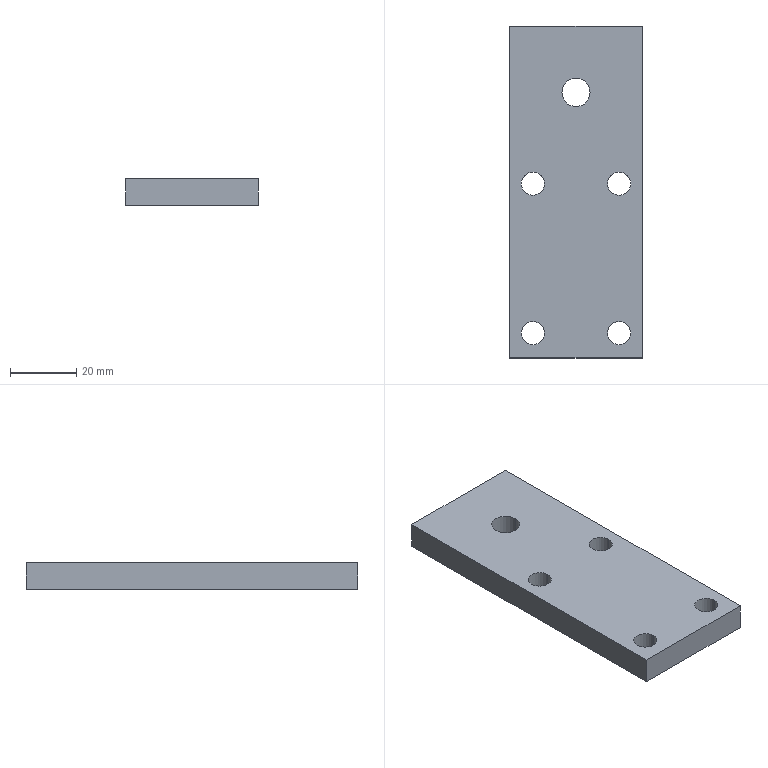Part | STEP file | X77-03028 | 1 solid | 16 faces | box 40 x 100 x 8 mm | volume 30315 mm3 | cylinder 10 | plane 6 | commonest cylinder face diameters 7 x8 8.5 x2
STEP:
#1=CARTESIAN_POINT('',(-1250.203,-4407.704,0.));
#2=VERTEX_POINT('',#1);
#3=CARTESIAN_POINT('',(-1258.703,-4407.704,0.));
#4=VERTEX_POINT('',#3);
#5=CARTESIAN_POINT('',(-1254.453,-4407.704,0.));
#6=DIRECTION('',(0.,0.,-1.));
#7=DIRECTION('',(-1.,0.,0.));
#8=AXIS2_PLACEMENT_3D('',#5,#6,#7);
#9=CIRCLE('',#8,4.25);
#10=EDGE_CURVE('',#2,#4,#9,.T.);
#11=ORIENTED_EDGE('',*,*,#10,.T.);
#12=CARTESIAN_POINT('',(-1258.703,-4407.704,8.));
#13=VERTEX_POINT('',#12);
#14=CARTESIAN_POINT('',(-1258.703,-4407.704,8.));
#15=DIRECTION('',(0.,0.,1.));
#16=VECTOR('',#15,1000.);
#17=LINE('',#14,#16);
#18=EDGE_CURVE('',#4,#13,#17,.T.);
#19=ORIENTED_EDGE('',*,*,#18,.T.);
#20=CARTESIAN_POINT('',(-1250.203,-4407.704,8.));
#21=VERTEX_POINT('',#20);
#22=CARTESIAN_POINT('',(-1254.453,-4407.704,8.));
#23=DIRECTION('',(0.,0.,1.));
#24=DIRECTION('',(1.,0.,0.));
#25=AXIS2_PLACEMENT_3D('',#22,#23,#24);
#26=CIRCLE('',#25,4.25);
#27=EDGE_CURVE('',#13,#21,#26,.T.);
#28=ORIENTED_EDGE('',*,*,#27,.T.);
#29=CARTESIAN_POINT('',(-1250.203,-4407.704,8.));
#30=DIRECTION('',(0.,0.,1.));
#31=VECTOR('',#30,1000.);
#32=LINE('',#29,#31);
#33=EDGE_CURVE('',#2,#21,#32,.T.);
#34=ORIENTED_EDGE('',*,*,#33,.F.);
#35=EDGE_LOOP('',(#11,#19,#28,#34));
#36=FACE_OUTER_BOUND('',#35,.T.);
#37=CARTESIAN_POINT('',(-1254.453,-4407.704,8.));
#38=DIRECTION('',(0.,0.,1.));
#39=DIRECTION('',(1.,0.,0.));
#40=AXIS2_PLACEMENT_3D('',#37,#38,#39);
#41=CYLINDRICAL_SURFACE('',#40,4.25);
#42=ADVANCED_FACE('',(#36),#41,.F.);
#43=CARTESIAN_POINT('',(-1244.953,-4480.204,8.));
#44=VERTEX_POINT('',#43);
#45=CARTESIAN_POINT('',(-1237.953,-4480.204,8.));
#46=VERTEX_POINT('',#45);
#47=CARTESIAN_POINT('',(-1241.453,-4480.204,8.));
#48=DIRECTION('',(0.,0.,1.));
#49=DIRECTION('',(1.,0.,0.));
#50=AXIS2_PLACEMENT_3D('',#47,#48,#49);
#51=CIRCLE('',#50,3.5);
#52=EDGE_CURVE('',#44,#46,#51,.T.);
#53=ORIENTED_EDGE('',*,*,#52,.T.);
#54=CARTESIAN_POINT('',(-1237.953,-4480.204,0.));
#55=VERTEX_POINT('',#54);
#56=CARTESIAN_POINT('',(-1237.953,-4480.204,8.));
#57=DIRECTION('',(0.,0.,-1.));
#58=VECTOR('',#57,1000.);
#59=LINE('',#56,#58);
#60=EDGE_CURVE('',#46,#55,#59,.T.);
#61=ORIENTED_EDGE('',*,*,#60,.T.);
#62=CARTESIAN_POINT('',(-1244.953,-4480.204,0.));
#63=VERTEX_POINT('',#62);
#64=CARTESIAN_POINT('',(-1241.453,-4480.204,0.));
#65=DIRECTION('',(0.,0.,1.));
#66=DIRECTION('',(1.,0.,0.));
#67=AXIS2_PLACEMENT_3D('',#64,#65,#66);
#68=CIRCLE('',#67,3.5);
#69=EDGE_CURVE('',#63,#55,#68,.T.);
#70=ORIENTED_EDGE('',*,*,#69,.F.);
#71=CARTESIAN_POINT('',(-1244.953,-4480.204,8.));
#72=DIRECTION('',(0.,0.,-1.));
#73=VECTOR('',#72,1000.);
#74=LINE('',#71,#73);
#75=EDGE_CURVE('',#44,#63,#74,.T.);
#76=ORIENTED_EDGE('',*,*,#75,.F.);
#77=EDGE_LOOP('',(#53,#61,#70,#76));
#78=FACE_OUTER_BOUND('',#77,.T.);
#79=CARTESIAN_POINT('',(-1241.453,-4480.204,8.));
#80=DIRECTION('',(0.,0.,-1.));
#81=DIRECTION('',(-1.,0.,0.));
#82=AXIS2_PLACEMENT_3D('',#79,#80,#81);
#83=CYLINDRICAL_SURFACE('',#82,3.5);
#84=ADVANCED_FACE('',(#78),#83,.F.);
#85=CARTESIAN_POINT('',(-1270.953,-4480.204,8.));
#86=VERTEX_POINT('',#85);
#87=CARTESIAN_POINT('',(-1263.953,-4480.204,8.));
#88=VERTEX_POINT('',#87);
#89=CARTESIAN_POINT('',(-1267.453,-4480.204,8.));
#90=DIRECTION('',(0.,0.,1.));
#91=DIRECTION('',(1.,0.,0.));
#92=AXIS2_PLACEMENT_3D('',#89,#90,#91);
#93=CIRCLE('',#92,3.5);
#94=EDGE_CURVE('',#86,#88,#93,.T.);
#95=ORIENTED_EDGE('',*,*,#94,.T.);
#96=CARTESIAN_POINT('',(-1263.953,-4480.204,0.));
#97=VERTEX_POINT('',#96);
#98=CARTESIAN_POINT('',(-1263.953,-4480.204,8.));
#99=DIRECTION('',(0.,0.,-1.));
#100=VECTOR('',#99,1000.);
#101=LINE('',#98,#100);
#102=EDGE_CURVE('',#88,#97,#101,.T.);
#103=ORIENTED_EDGE('',*,*,#102,.T.);
#104=CARTESIAN_POINT('',(-1270.953,-4480.204,0.));
#105=VERTEX_POINT('',#104);
#106=CARTESIAN_POINT('',(-1267.453,-4480.204,0.));
#107=DIRECTION('',(0.,0.,1.));
#108=DIRECTION('',(1.,0.,0.));
#109=AXIS2_PLACEMENT_3D('',#106,#107,#108);
#110=CIRCLE('',#109,3.5);
#111=EDGE_CURVE('',#105,#97,#110,.T.);
#112=ORIENTED_EDGE('',*,*,#111,.F.);
#113=CARTESIAN_POINT('',(-1270.953,-4480.204,8.));
#114=DIRECTION('',(0.,0.,-1.));
#115=VECTOR('',#114,1000.);
#116=LINE('',#113,#115);
#117=EDGE_CURVE('',#86,#105,#116,.T.);
#118=ORIENTED_EDGE('',*,*,#117,.F.);
#119=EDGE_LOOP('',(#95,#103,#112,#118));
#120=FACE_OUTER_BOUND('',#119,.T.);
#121=CARTESIAN_POINT('',(-1267.453,-4480.204,8.));
#122=DIRECTION('',(0.,0.,-1.));
#123=DIRECTION('',(-1.,0.,0.));
#124=AXIS2_PLACEMENT_3D('',#121,#122,#123);
#125=CYLINDRICAL_SURFACE('',#124,3.5);
#126=ADVANCED_FACE('',(#120),#125,.F.);
#127=CARTESIAN_POINT('',(-1244.953,-4435.204,8.));
#128=VERTEX_POINT('',#127);
#129=CARTESIAN_POINT('',(-1237.953,-4435.204,8.));
#130=VERTEX_POINT('',#129);
#131=CARTESIAN_POINT('',(-1241.453,-4435.204,8.));
#132=DIRECTION('',(0.,0.,1.));
#133=DIRECTION('',(1.,0.,0.));
#134=AXIS2_PLACEMENT_3D('',#131,#132,#133);
#135=CIRCLE('',#134,3.5);
#136=EDGE_CURVE('',#128,#130,#135,.T.);
#137=ORIENTED_EDGE('',*,*,#136,.T.);
#138=CARTESIAN_POINT('',(-1237.953,-4435.204,0.));
#139=VERTEX_POINT('',#138);
#140=CARTESIAN_POINT('',(-1237.953,-4435.204,8.));
#141=DIRECTION('',(0.,0.,-1.));
#142=VECTOR('',#141,1000.);
#143=LINE('',#140,#142);
#144=EDGE_CURVE('',#130,#139,#143,.T.);
#145=ORIENTED_EDGE('',*,*,#144,.T.);
#146=CARTESIAN_POINT('',(-1244.953,-4435.204,0.));
#147=VERTEX_POINT('',#146);
#148=CARTESIAN_POINT('',(-1241.453,-4435.204,0.));
#149=DIRECTION('',(0.,0.,1.));
#150=DIRECTION('',(1.,0.,0.));
#151=AXIS2_PLACEMENT_3D('',#148,#149,#150);
#152=CIRCLE('',#151,3.5);
#153=EDGE_CURVE('',#147,#139,#152,.T.);
#154=ORIENTED_EDGE('',*,*,#153,.F.);
#155=CARTESIAN_POINT('',(-1244.953,-4435.204,8.));
#156=DIRECTION('',(0.,0.,-1.));
#157=VECTOR('',#156,1000.);
#158=LINE('',#155,#157);
#159=EDGE_CURVE('',#128,#147,#158,.T.);
#160=ORIENTED_EDGE('',*,*,#159,.F.);
#161=EDGE_LOOP('',(#137,#145,#154,#160));
#162=FACE_OUTER_BOUND('',#161,.T.);
#163=CARTESIAN_POINT('',(-1241.453,-4435.204,8.));
#164=DIRECTION('',(0.,0.,-1.));
#165=DIRECTION('',(-1.,0.,0.));
#166=AXIS2_PLACEMENT_3D('',#163,#164,#165);
#167=CYLINDRICAL_SURFACE('',#166,3.5);
#168=ADVANCED_FACE('',(#162),#167,.F.);
#169=CARTESIAN_POINT('',(-1270.953,-4435.204,8.));
#170=VERTEX_POINT('',#169);
#171=CARTESIAN_POINT('',(-1263.953,-4435.204,8.));
#172=VERTEX_POINT('',#171);
#173=CARTESIAN_POINT('',(-1267.453,-4435.204,8.));
#174=DIRECTION('',(0.,0.,1.));
#175=DIRECTION('',(1.,0.,0.));
#176=AXIS2_PLACEMENT_3D('',#173,#174,#175);
#177=CIRCLE('',#176,3.5);
#178=EDGE_CURVE('',#170,#172,#177,.T.);
#179=ORIENTED_EDGE('',*,*,#178,.T.);
#180=CARTESIAN_POINT('',(-1263.953,-4435.204,0.));
#181=VERTEX_POINT('',#180);
#182=CARTESIAN_POINT('',(-1263.953,-4435.204,8.));
#183=DIRECTION('',(0.,0.,-1.));
#184=VECTOR('',#183,1000.);
#185=LINE('',#182,#184);
#186=EDGE_CURVE('',#172,#181,#185,.T.);
#187=ORIENTED_EDGE('',*,*,#186,.T.);
#188=CARTESIAN_POINT('',(-1270.953,-4435.204,0.));
#189=VERTEX_POINT('',#188);
#190=CARTESIAN_POINT('',(-1267.453,-4435.204,0.));
#191=DIRECTION('',(0.,0.,1.));
#192=DIRECTION('',(1.,0.,0.));
#193=AXIS2_PLACEMENT_3D('',#190,#191,#192);
#194=CIRCLE('',#193,3.5);
#195=EDGE_CURVE('',#189,#181,#194,.T.);
#196=ORIENTED_EDGE('',*,*,#195,.F.);
#197=CARTESIAN_POINT('',(-1270.953,-4435.204,8.));
#198=DIRECTION('',(0.,0.,-1.));
#199=VECTOR('',#198,1000.);
#200=LINE('',#197,#199);
#201=EDGE_CURVE('',#170,#189,#200,.T.);
#202=ORIENTED_EDGE('',*,*,#201,.F.);
#203=EDGE_LOOP('',(#179,#187,#196,#202));
#204=FACE_OUTER_BOUND('',#203,.T.);
#205=CARTESIAN_POINT('',(-1267.453,-4435.204,8.));
#206=DIRECTION('',(0.,0.,-1.));
#207=DIRECTION('',(-1.,0.,0.));
#208=AXIS2_PLACEMENT_3D('',#205,#206,#207);
#209=CYLINDRICAL_SURFACE('',#208,3.5);
#210=ADVANCED_FACE('',(#204),#209,.F.);
#211=CARTESIAN_POINT('',(-1254.453,-4407.704,8.));
#212=DIRECTION('',(0.,0.,1.));
#213=DIRECTION('',(1.,0.,0.));
#214=AXIS2_PLACEMENT_3D('',#211,#212,#213);
#215=CIRCLE('',#214,4.25);
#216=EDGE_CURVE('',#21,#13,#215,.T.);
#217=ORIENTED_EDGE('',*,*,#216,.F.);
#218=ORIENTED_EDGE('',*,*,#27,.F.);
#219=EDGE_LOOP('',(#217,#218));
#220=FACE_BOUND('',#219,.T.);
#221=ORIENTED_EDGE('',*,*,#94,.F.);
#222=CARTESIAN_POINT('',(-1267.453,-4480.204,8.));
#223=DIRECTION('',(0.,0.,1.));
#224=DIRECTION('',(1.,0.,0.));
#225=AXIS2_PLACEMENT_3D('',#222,#223,#224);
#226=CIRCLE('',#225,3.5);
#227=EDGE_CURVE('',#88,#86,#226,.T.);
#228=ORIENTED_EDGE('',*,*,#227,.F.);
#229=EDGE_LOOP('',(#221,#228));
#230=FACE_BOUND('',#229,.T.);
#231=ORIENTED_EDGE('',*,*,#178,.F.);
#232=CARTESIAN_POINT('',(-1267.453,-4435.204,8.));
#233=DIRECTION('',(0.,0.,1.));
#234=DIRECTION('',(1.,0.,0.));
#235=AXIS2_PLACEMENT_3D('',#232,#233,#234);
#236=CIRCLE('',#235,3.5);
#237=EDGE_CURVE('',#172,#170,#236,.T.);
#238=ORIENTED_EDGE('',*,*,#237,.F.);
#239=EDGE_LOOP('',(#231,#238));
#240=FACE_BOUND('',#239,.T.);
#241=CARTESIAN_POINT('',(-1234.453,-4487.704,8.));
#242=VERTEX_POINT('',#241);
#243=CARTESIAN_POINT('',(-1234.453,-4387.704,8.));
#244=VERTEX_POINT('',#243);
#245=CARTESIAN_POINT('',(-1234.453,-4487.704,8.));
#246=DIRECTION('',(0.,1.,0.));
#247=VECTOR('',#246,1000.);
#248=LINE('',#245,#247);
#249=EDGE_CURVE('',#242,#244,#248,.T.);
#250=ORIENTED_EDGE('',*,*,#249,.T.);
#251=CARTESIAN_POINT('',(-1274.453,-4387.704,8.));
#252=VERTEX_POINT('',#251);
#253=CARTESIAN_POINT('',(-1274.453,-4387.704,8.));
#254=DIRECTION('',(-1.,0.,0.));
#255=VECTOR('',#254,1000.);
#256=LINE('',#253,#255);
#257=EDGE_CURVE('',#244,#252,#256,.T.);
#258=ORIENTED_EDGE('',*,*,#257,.T.);
#259=CARTESIAN_POINT('',(-1274.453,-4487.704,8.));
#260=VERTEX_POINT('',#259);
#261=CARTESIAN_POINT('',(-1274.453,-4487.704,8.));
#262=DIRECTION('',(0.,-1.,0.));
#263=VECTOR('',#262,1000.);
#264=LINE('',#261,#263);
#265=EDGE_CURVE('',#252,#260,#264,.T.);
#266=ORIENTED_EDGE('',*,*,#265,.T.);
#267=CARTESIAN_POINT('',(-1274.453,-4487.704,8.));
#268=DIRECTION('',(1.,0.,0.));
#269=VECTOR('',#268,1000.);
#270=LINE('',#267,#269);
#271=EDGE_CURVE('',#260,#242,#270,.T.);
#272=ORIENTED_EDGE('',*,*,#271,.T.);
#273=EDGE_LOOP('',(#250,#258,#266,#272));
#274=FACE_OUTER_BOUND('',#273,.T.);
#275=ORIENTED_EDGE('',*,*,#136,.F.);
#276=CARTESIAN_POINT('',(-1241.453,-4435.204,8.));
#277=DIRECTION('',(0.,0.,1.));
#278=DIRECTION('',(1.,0.,0.));
#279=AXIS2_PLACEMENT_3D('',#276,#277,#278);
#280=CIRCLE('',#279,3.5);
#281=EDGE_CURVE('',#130,#128,#280,.T.);
#282=ORIENTED_EDGE('',*,*,#281,.F.);
#283=EDGE_LOOP('',(#275,#282));
#284=FACE_BOUND('',#283,.T.);
#285=ORIENTED_EDGE('',*,*,#52,.F.);
#286=CARTESIAN_POINT('',(-1241.453,-4480.204,8.));
#287=DIRECTION('',(0.,0.,1.));
#288=DIRECTION('',(1.,0.,0.));
#289=AXIS2_PLACEMENT_3D('',#286,#287,#288);
#290=CIRCLE('',#289,3.5);
#291=EDGE_CURVE('',#46,#44,#290,.T.);
#292=ORIENTED_EDGE('',*,*,#291,.F.);
#293=EDGE_LOOP('',(#285,#292));
#294=FACE_BOUND('',#293,.T.);
#295=CARTESIAN_POINT('',(-1234.453,-4387.704,8.));
#296=DIRECTION('',(0.,0.,-1.));
#297=DIRECTION('',(-1.,0.,0.));
#298=AXIS2_PLACEMENT_3D('',#295,#296,#297);
#299=PLANE('',#298);
#300=ADVANCED_FACE('',(#220,#230,#240,#274,#284,#294),#299,.F.);
#301=ORIENTED_EDGE('',*,*,#10,.F.);
#302=CARTESIAN_POINT('',(-1254.453,-4407.704,0.));
#303=DIRECTION('',(0.,0.,-1.));
#304=DIRECTION('',(-1.,0.,0.));
#305=AXIS2_PLACEMENT_3D('',#302,#303,#304);
#306=CIRCLE('',#305,4.25);
#307=EDGE_CURVE('',#4,#2,#306,.T.);
#308=ORIENTED_EDGE('',*,*,#307,.F.);
#309=EDGE_LOOP('',(#301,#308));
#310=FACE_BOUND('',#309,.T.);
#311=ORIENTED_EDGE('',*,*,#111,.T.);
#312=CARTESIAN_POINT('',(-1267.453,-4480.204,0.));
#313=DIRECTION('',(0.,0.,1.));
#314=DIRECTION('',(1.,0.,0.));
#315=AXIS2_PLACEMENT_3D('',#312,#313,#314);
#316=CIRCLE('',#315,3.5);
#317=EDGE_CURVE('',#97,#105,#316,.T.);
#318=ORIENTED_EDGE('',*,*,#317,.T.);
#319=EDGE_LOOP('',(#311,#318));
#320=FACE_BOUND('',#319,.T.);
#321=ORIENTED_EDGE('',*,*,#195,.T.);
#322=CARTESIAN_POINT('',(-1267.453,-4435.204,0.));
#323=DIRECTION('',(0.,0.,1.));
#324=DIRECTION('',(1.,0.,0.));
#325=AXIS2_PLACEMENT_3D('',#322,#323,#324);
#326=CIRCLE('',#325,3.5);
#327=EDGE_CURVE('',#181,#189,#326,.T.);
#328=ORIENTED_EDGE('',*,*,#327,.T.);
#329=EDGE_LOOP('',(#321,#328));
#330=FACE_BOUND('',#329,.T.);
#331=CARTESIAN_POINT('',(-1234.453,-4487.704,0.));
#332=VERTEX_POINT('',#331);
#333=CARTESIAN_POINT('',(-1234.453,-4387.704,0.));
#334=VERTEX_POINT('',#333);
#335=CARTESIAN_POINT('',(-1234.453,-4487.704,0.));
#336=DIRECTION('',(0.,1.,0.));
#337=VECTOR('',#336,1000.);
#338=LINE('',#335,#337);
#339=EDGE_CURVE('',#332,#334,#338,.T.);
#340=ORIENTED_EDGE('',*,*,#339,.F.);
#341=CARTESIAN_POINT('',(-1274.453,-4487.704,0.));
#342=VERTEX_POINT('',#341);
#343=CARTESIAN_POINT('',(-1274.453,-4487.704,0.));
#344=DIRECTION('',(1.,0.,0.));
#345=VECTOR('',#344,1000.);
#346=LINE('',#343,#345);
#347=EDGE_CURVE('',#342,#332,#346,.T.);
#348=ORIENTED_EDGE('',*,*,#347,.F.);
#349=CARTESIAN_POINT('',(-1274.453,-4387.704,0.));
#350=VERTEX_POINT('',#349);
#351=CARTESIAN_POINT('',(-1274.453,-4487.704,0.));
#352=DIRECTION('',(0.,-1.,0.));
#353=VECTOR('',#352,1000.);
#354=LINE('',#351,#353);
#355=EDGE_CURVE('',#350,#342,#354,.T.);
#356=ORIENTED_EDGE('',*,*,#355,.F.);
#357=CARTESIAN_POINT('',(-1274.453,-4387.704,0.));
#358=DIRECTION('',(-1.,0.,0.));
#359=VECTOR('',#358,1000.);
#360=LINE('',#357,#359);
#361=EDGE_CURVE('',#334,#350,#360,.T.);
#362=ORIENTED_EDGE('',*,*,#361,.F.);
#363=EDGE_LOOP('',(#340,#348,#356,#362));
#364=FACE_OUTER_BOUND('',#363,.T.);
#365=ORIENTED_EDGE('',*,*,#153,.T.);
#366=CARTESIAN_POINT('',(-1241.453,-4435.204,0.));
#367=DIRECTION('',(0.,0.,1.));
#368=DIRECTION('',(1.,0.,0.));
#369=AXIS2_PLACEMENT_3D('',#366,#367,#368);
#370=CIRCLE('',#369,3.5);
#371=EDGE_CURVE('',#139,#147,#370,.T.);
#372=ORIENTED_EDGE('',*,*,#371,.T.);
#373=EDGE_LOOP('',(#365,#372));
#374=FACE_BOUND('',#373,.T.);
#375=ORIENTED_EDGE('',*,*,#69,.T.);
#376=CARTESIAN_POINT('',(-1241.453,-4480.204,0.));
#377=DIRECTION('',(0.,0.,1.));
#378=DIRECTION('',(1.,0.,0.));
#379=AXIS2_PLACEMENT_3D('',#376,#377,#378);
#380=CIRCLE('',#379,3.5);
#381=EDGE_CURVE('',#55,#63,#380,.T.);
#382=ORIENTED_EDGE('',*,*,#381,.T.);
#383=EDGE_LOOP('',(#375,#382));
#384=FACE_BOUND('',#383,.T.);
#385=CARTESIAN_POINT('',(-1234.453,-4387.704,0.));
#386=DIRECTION('',(0.,0.,-1.));
#387=DIRECTION('',(-1.,0.,0.));
#388=AXIS2_PLACEMENT_3D('',#385,#386,#387);
#389=PLANE('',#388);
#390=ADVANCED_FACE('',(#310,#320,#330,#364,#374,#384),#389,.T.);
#391=ORIENTED_EDGE('',*,*,#339,.T.);
#392=CARTESIAN_POINT('',(-1234.453,-4387.704,8.));
#393=DIRECTION('',(0.,0.,-1.));
#394=VECTOR('',#393,1000.);
#395=LINE('',#392,#394);
#396=EDGE_CURVE('',#244,#334,#395,.T.);
#397=ORIENTED_EDGE('',*,*,#396,.F.);
#398=ORIENTED_EDGE('',*,*,#249,.F.);
#399=CARTESIAN_POINT('',(-1234.453,-4487.704,8.));
#400=DIRECTION('',(0.,0.,-1.));
#401=VECTOR('',#400,1000.);
#402=LINE('',#399,#401);
#403=EDGE_CURVE('',#242,#332,#402,.T.);
#404=ORIENTED_EDGE('',*,*,#403,.T.);
#405=EDGE_LOOP('',(#391,#397,#398,#404));
#406=FACE_OUTER_BOUND('',#405,.T.);
#407=CARTESIAN_POINT('',(-1234.453,-4487.704,8.));
#408=DIRECTION('',(-1.,0.,0.));
#409=DIRECTION('',(0.,0.,1.));
#410=AXIS2_PLACEMENT_3D('',#407,#408,#409);
#411=PLANE('',#410);
#412=ADVANCED_FACE('',(#406),#411,.F.);
#413=ORIENTED_EDGE('',*,*,#361,.T.);
#414=CARTESIAN_POINT('',(-1274.453,-4387.704,8.));
#415=DIRECTION('',(0.,0.,-1.));
#416=VECTOR('',#415,1000.);
#417=LINE('',#414,#416);
#418=EDGE_CURVE('',#252,#350,#417,.T.);
#419=ORIENTED_EDGE('',*,*,#418,.F.);
#420=ORIENTED_EDGE('',*,*,#257,.F.);
#421=ORIENTED_EDGE('',*,*,#396,.T.);
#422=EDGE_LOOP('',(#413,#419,#420,#421));
#423=FACE_OUTER_BOUND('',#422,.T.);
#424=CARTESIAN_POINT('',(-1274.453,-4387.704,8.));
#425=DIRECTION('',(0.,-1.,0.));
#426=DIRECTION('',(0.,0.,-1.));
#427=AXIS2_PLACEMENT_3D('',#424,#425,#426);
#428=PLANE('',#427);
#429=ADVANCED_FACE('',(#423),#428,.F.);
#430=ORIENTED_EDGE('',*,*,#355,.T.);
#431=CARTESIAN_POINT('',(-1274.453,-4487.704,8.));
#432=DIRECTION('',(0.,0.,-1.));
#433=VECTOR('',#432,1000.);
#434=LINE('',#431,#433);
#435=EDGE_CURVE('',#260,#342,#434,.T.);
#436=ORIENTED_EDGE('',*,*,#435,.F.);
#437=ORIENTED_EDGE('',*,*,#265,.F.);
#438=ORIENTED_EDGE('',*,*,#418,.T.);
#439=EDGE_LOOP('',(#430,#436,#437,#438));
#440=FACE_OUTER_BOUND('',#439,.T.);
#441=CARTESIAN_POINT('',(-1274.453,-4487.704,8.));
#442=DIRECTION('',(1.,0.,0.));
#443=DIRECTION('',(0.,0.,-1.));
#444=AXIS2_PLACEMENT_3D('',#441,#442,#443);
#445=PLANE('',#444);
#446=ADVANCED_FACE('',(#440),#445,.F.);
#447=ORIENTED_EDGE('',*,*,#347,.T.);
#448=ORIENTED_EDGE('',*,*,#403,.F.);
#449=ORIENTED_EDGE('',*,*,#271,.F.);
#450=ORIENTED_EDGE('',*,*,#435,.T.);
#451=EDGE_LOOP('',(#447,#448,#449,#450));
#452=FACE_OUTER_BOUND('',#451,.T.);
#453=CARTESIAN_POINT('',(-1274.453,-4487.704,8.));
#454=DIRECTION('',(0.,1.,0.));
#455=DIRECTION('',(0.,0.,1.));
#456=AXIS2_PLACEMENT_3D('',#453,#454,#455);
#457=PLANE('',#456);
#458=ADVANCED_FACE('',(#452),#457,.F.);
#459=ORIENTED_EDGE('',*,*,#186,.F.);
#460=ORIENTED_EDGE('',*,*,#237,.T.);
#461=ORIENTED_EDGE('',*,*,#201,.T.);
#462=ORIENTED_EDGE('',*,*,#327,.F.);
#463=EDGE_LOOP('',(#459,#460,#461,#462));
#464=FACE_OUTER_BOUND('',#463,.T.);
#465=CARTESIAN_POINT('',(-1267.453,-4435.204,8.));
#466=DIRECTION('',(0.,0.,-1.));
#467=DIRECTION('',(-1.,0.,0.));
#468=AXIS2_PLACEMENT_3D('',#465,#466,#467);
#469=CYLINDRICAL_SURFACE('',#468,3.5);
#470=ADVANCED_FACE('',(#464),#469,.F.);
#471=ORIENTED_EDGE('',*,*,#144,.F.);
#472=ORIENTED_EDGE('',*,*,#281,.T.);
#473=ORIENTED_EDGE('',*,*,#159,.T.);
#474=ORIENTED_EDGE('',*,*,#371,.F.);
#475=EDGE_LOOP('',(#471,#472,#473,#474));
#476=FACE_OUTER_BOUND('',#475,.T.);
#477=CARTESIAN_POINT('',(-1241.453,-4435.204,8.));
#478=DIRECTION('',(0.,0.,-1.));
#479=DIRECTION('',(-1.,0.,0.));
#480=AXIS2_PLACEMENT_3D('',#477,#478,#479);
#481=CYLINDRICAL_SURFACE('',#480,3.5);
#482=ADVANCED_FACE('',(#476),#481,.F.);
#483=ORIENTED_EDGE('',*,*,#102,.F.);
#484=ORIENTED_EDGE('',*,*,#227,.T.);
#485=ORIENTED_EDGE('',*,*,#117,.T.);
#486=ORIENTED_EDGE('',*,*,#317,.F.);
#487=EDGE_LOOP('',(#483,#484,#485,#486));
#488=FACE_OUTER_BOUND('',#487,.T.);
#489=CARTESIAN_POINT('',(-1267.453,-4480.204,8.));
#490=DIRECTION('',(0.,0.,-1.));
#491=DIRECTION('',(-1.,0.,0.));
#492=AXIS2_PLACEMENT_3D('',#489,#490,#491);
#493=CYLINDRICAL_SURFACE('',#492,3.5);
#494=ADVANCED_FACE('',(#488),#493,.F.);
#495=ORIENTED_EDGE('',*,*,#60,.F.);
#496=ORIENTED_EDGE('',*,*,#291,.T.);
#497=ORIENTED_EDGE('',*,*,#75,.T.);
#498=ORIENTED_EDGE('',*,*,#381,.F.);
#499=EDGE_LOOP('',(#495,#496,#497,#498));
#500=FACE_OUTER_BOUND('',#499,.T.);
#501=CARTESIAN_POINT('',(-1241.453,-4480.204,8.));
#502=DIRECTION('',(0.,0.,-1.));
#503=DIRECTION('',(-1.,0.,0.));
#504=AXIS2_PLACEMENT_3D('',#501,#502,#503);
#505=CYLINDRICAL_SURFACE('',#504,3.5);
#506=ADVANCED_FACE('',(#500),#505,.F.);
#507=ORIENTED_EDGE('',*,*,#18,.F.);
#508=ORIENTED_EDGE('',*,*,#307,.T.);
#509=ORIENTED_EDGE('',*,*,#33,.T.);
#510=ORIENTED_EDGE('',*,*,#216,.T.);
#511=EDGE_LOOP('',(#507,#508,#509,#510));
#512=FACE_OUTER_BOUND('',#511,.T.);
#513=CARTESIAN_POINT('',(-1254.453,-4407.704,8.));
#514=DIRECTION('',(0.,0.,1.));
#515=DIRECTION('',(1.,0.,0.));
#516=AXIS2_PLACEMENT_3D('',#513,#514,#515);
#517=CYLINDRICAL_SURFACE('',#516,4.25);
#518=ADVANCED_FACE('',(#512),#517,.F.);
#519=CLOSED_SHELL('',(#42,#84,#126,#168,#210,#300,#390,#412,#429,#446,#458,#470,#482,#494,#506,#518));
#520=MANIFOLD_SOLID_BREP('',#519);
#521=CARTESIAN_POINT('',(0.,0.,0.));
#522=DIRECTION('',(0.,0.,1.));
#523=DIRECTION('',(1.,0.,0.));
#524=AXIS2_PLACEMENT_3D('',#521,#522,#523);
#525=(LENGTH_UNIT()NAMED_UNIT(*)SI_UNIT(.MILLI.,.METRE.));
#526=UNCERTAINTY_MEASURE_WITH_UNIT(LENGTH_MEASURE(0.00001),#525,'','');
#527=(NAMED_UNIT(*)PLANE_ANGLE_UNIT()SI_UNIT($,.RADIAN.));
#528=(NAMED_UNIT(*)SI_UNIT($,.STERADIAN.)SOLID_ANGLE_UNIT());
#529=(GEOMETRIC_REPRESENTATION_CONTEXT(3)GLOBAL_UNCERTAINTY_ASSIGNED_CONTEXT((#526))GLOBAL_UNIT_ASSIGNED_CONTEXT((#525,#527,#528))REPRESENTATION_CONTEXT('',''));
#530=ADVANCED_BREP_SHAPE_REPRESENTATION('',(#520,#524),#529);